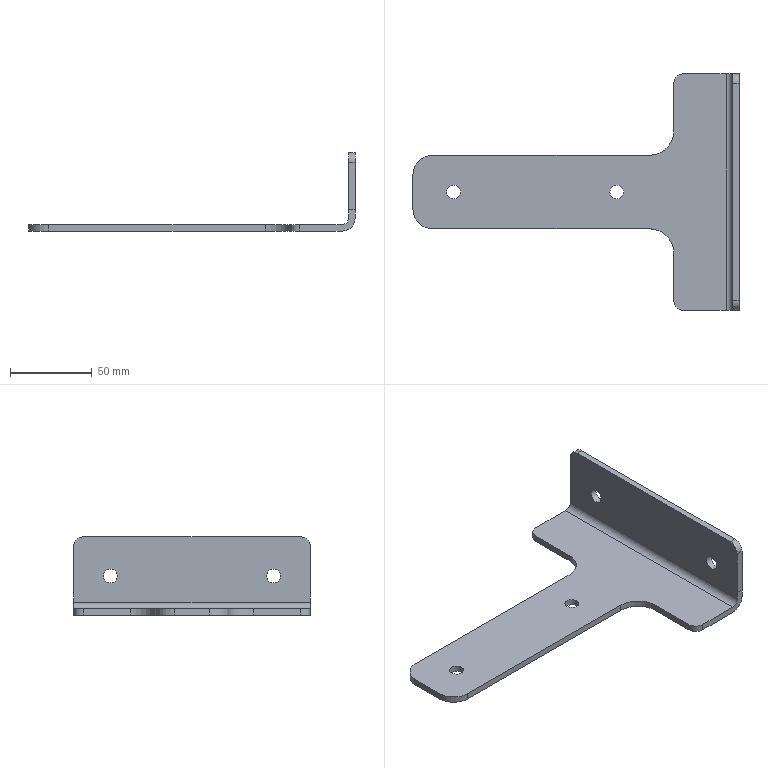Part | STEP file | Connector TR lift wer2 | 1 solid | 28 faces | box 200 x 145 x 48 mm | volume 75134 mm3 | cylinder 14 | plane 14 | commonest cylinder face diameters 8.5 x4 12 x4 24 x2 30 x2 8 x1 16 x1